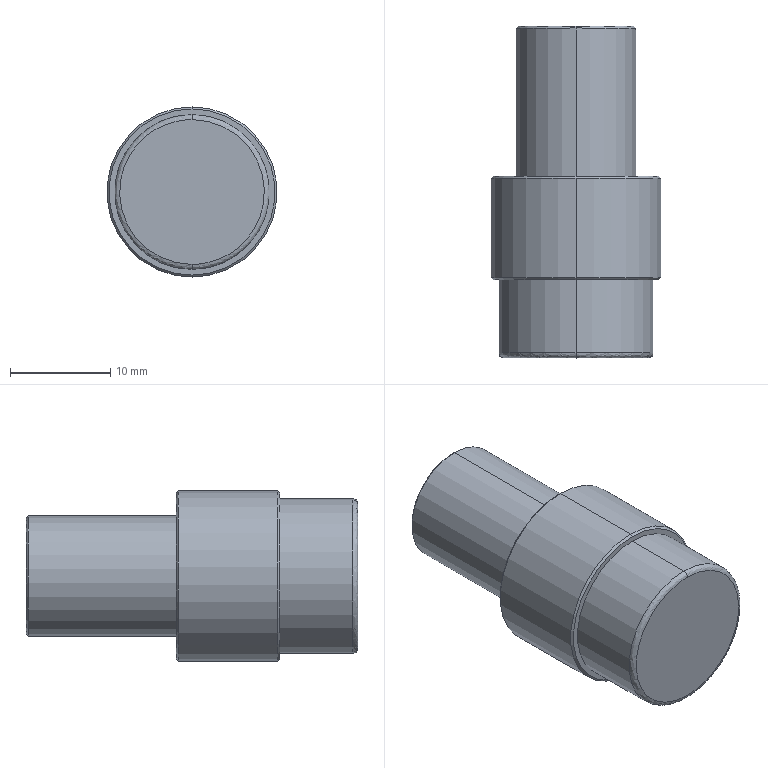Part | SolidWorks | features BaseBody 1 | 1 solid | 18 faces | box 17 x 33.14 x 17 mm | volume 5502 mm3 | cylinder 6 | cone 6 | plane 4 | spline 2 | commonest cylinder face diameters 12 x2 15.46 x2 17 x2
STEP:
#1=CARTESIAN_POINT('',(0.,0.5,-7.73));
#2=VERTEX_POINT('',#1);
#3=CARTESIAN_POINT('',(0.,0.5,7.73));
#4=VERTEX_POINT('',#3);
#5=CARTESIAN_POINT('',(0.,0.5,0.));
#6=DIRECTION('',(0.,1.,0.));
#7=DIRECTION('',(0.,0.,-1.));
#8=AXIS2_PLACEMENT_3D('',#5,#6,#7);
#9=CIRCLE('',#8,7.73);
#10=EDGE_CURVE('',#2,#4,#9,.T.);
#11=ORIENTED_EDGE('',*,*,#10,.F.);
#12=CARTESIAN_POINT('',(0.,0.,-7.23));
#13=VERTEX_POINT('',#12);
#14=CARTESIAN_POINT('',(0.,0.5,-7.23));
#15=DIRECTION('',(-1.,0.,0.));
#16=DIRECTION('',(0.,0.,-1.));
#17=AXIS2_PLACEMENT_3D('',#14,#15,#16);
#18=CIRCLE('',#17,0.5);
#19=EDGE_CURVE('',#2,#13,#18,.T.);
#20=ORIENTED_EDGE('',*,*,#19,.T.);
#21=CARTESIAN_POINT('',(0.,0.,7.23));
#22=VERTEX_POINT('',#21);
#23=CARTESIAN_POINT('',(0.,0.,-7.23));
#24=CARTESIAN_POINT('',(-14.46,0.,-7.23));
#25=CARTESIAN_POINT('',(-14.46,0.,7.23));
#26=CARTESIAN_POINT('',(0.,0.,7.23));
#27=(BOUNDED_CURVE()B_SPLINE_CURVE(3,(#23,#24,#25,#26),.UNSPECIFIED.,.F.,.T.)B_SPLINE_CURVE_WITH_KNOTS((4,4),(0.,1.),.UNSPECIFIED.)CURVE()GEOMETRIC_REPRESENTATION_ITEM()RATIONAL_B_SPLINE_CURVE((1.,0.3333,0.3333,1.))REPRESENTATION_ITEM(''));
#28=EDGE_CURVE('',#13,#22,#27,.T.);
#29=ORIENTED_EDGE('',*,*,#28,.T.);
#30=CARTESIAN_POINT('',(0.,0.5,7.23));
#31=DIRECTION('',(1.,0.,0.));
#32=DIRECTION('',(0.,0.,1.));
#33=AXIS2_PLACEMENT_3D('',#30,#31,#32);
#34=CIRCLE('',#33,0.5);
#35=EDGE_CURVE('',#4,#22,#34,.T.);
#36=ORIENTED_EDGE('',*,*,#35,.F.);
#37=EDGE_LOOP('',(#11,#20,#29,#36));
#38=FACE_OUTER_BOUND('',#37,.T.);
#39=CARTESIAN_POINT('',(0.,0.5,-7.73));
#40=CARTESIAN_POINT('',(-15.46,0.5,-7.73));
#41=CARTESIAN_POINT('',(-15.46,0.5,7.73));
#42=CARTESIAN_POINT('',(0.,0.5,7.73));
#43=CARTESIAN_POINT('',(0.,0.2071,-7.73));
#44=CARTESIAN_POINT('',(-15.46,0.2071,-7.73));
#45=CARTESIAN_POINT('',(-15.46,0.2071,7.73));
#46=CARTESIAN_POINT('',(0.,0.2071,7.73));
#47=CARTESIAN_POINT('',(0.,0.,-7.523));
#48=CARTESIAN_POINT('',(-15.046,0.,-7.523));
#49=CARTESIAN_POINT('',(-15.046,0.,7.523));
#50=CARTESIAN_POINT('',(0.,0.,7.523));
#51=CARTESIAN_POINT('',(0.,0.,-7.23));
#52=CARTESIAN_POINT('',(-14.46,0.,-7.23));
#53=CARTESIAN_POINT('',(-14.46,0.,7.23));
#54=CARTESIAN_POINT('',(0.,0.,7.23));
#55=(BOUNDED_SURFACE()B_SPLINE_SURFACE(3,3,((#39,#40,#41,#42),(#43,#44,#45,#46),(#47,#48,#49,#50),(#51,#52,#53,#54)),.UNSPECIFIED.,.F.,.F.,.F.)B_SPLINE_SURFACE_WITH_KNOTS((4,4),(4,4),(0.,1.),(0.,1.),.UNSPECIFIED.)GEOMETRIC_REPRESENTATION_ITEM()RATIONAL_B_SPLINE_SURFACE(((1.,0.3333,0.3333,1.),(0.8047,0.2682,0.2682,0.8047),(0.8047,0.2682,0.2682,0.8047),(1.,0.3333,0.3333,1.)))REPRESENTATION_ITEM('')SURFACE());
#56=ADVANCED_FACE('',(#38),#55,.T.);
#57=CARTESIAN_POINT('',(0.,32.94,-6.));
#58=VERTEX_POINT('',#57);
#59=CARTESIAN_POINT('',(0.,32.94,6.));
#60=VERTEX_POINT('',#59);
#61=CARTESIAN_POINT('',(0.,32.94,0.));
#62=DIRECTION('',(0.,-1.,0.));
#63=DIRECTION('',(0.,0.,-1.));
#64=AXIS2_PLACEMENT_3D('',#61,#62,#63);
#65=CIRCLE('',#64,6.);
#66=EDGE_CURVE('',#58,#60,#65,.T.);
#67=ORIENTED_EDGE('',*,*,#66,.T.);
#68=CARTESIAN_POINT('',(0.,18.14,6.));
#69=VERTEX_POINT('',#68);
#70=CARTESIAN_POINT('',(0.,33.14,6.));
#71=DIRECTION('',(0.,-1.,0.));
#72=VECTOR('',#71,1000.);
#73=LINE('',#70,#72);
#74=EDGE_CURVE('',#60,#69,#73,.T.);
#75=ORIENTED_EDGE('',*,*,#74,.T.);
#76=CARTESIAN_POINT('',(0.,18.14,-6.));
#77=VERTEX_POINT('',#76);
#78=CARTESIAN_POINT('',(0.,18.14,0.));
#79=DIRECTION('',(0.,1.,0.));
#80=DIRECTION('',(0.,0.,-1.));
#81=AXIS2_PLACEMENT_3D('',#78,#79,#80);
#82=CIRCLE('',#81,6.);
#83=EDGE_CURVE('',#69,#77,#82,.T.);
#84=ORIENTED_EDGE('',*,*,#83,.T.);
#85=CARTESIAN_POINT('',(0.,33.14,-6.));
#86=DIRECTION('',(0.,-1.,0.));
#87=VECTOR('',#86,1000.);
#88=LINE('',#85,#87);
#89=EDGE_CURVE('',#58,#77,#88,.T.);
#90=ORIENTED_EDGE('',*,*,#89,.F.);
#91=EDGE_LOOP('',(#67,#75,#84,#90));
#92=FACE_OUTER_BOUND('',#91,.T.);
#93=CARTESIAN_POINT('',(0.,33.14,0.));
#94=DIRECTION('',(0.,-1.,0.));
#95=DIRECTION('',(0.,0.,-1.));
#96=AXIS2_PLACEMENT_3D('',#93,#94,#95);
#97=CYLINDRICAL_SURFACE('',#96,6.);
#98=ADVANCED_FACE('',(#92),#97,.T.);
#99=CARTESIAN_POINT('',(0.,33.14,-5.8));
#100=VERTEX_POINT('',#99);
#101=CARTESIAN_POINT('',(0.,33.14,5.8));
#102=VERTEX_POINT('',#101);
#103=CARTESIAN_POINT('',(0.,33.14,0.));
#104=DIRECTION('',(0.,-1.,0.));
#105=DIRECTION('',(0.,0.,-1.));
#106=AXIS2_PLACEMENT_3D('',#103,#104,#105);
#107=CIRCLE('',#106,5.8);
#108=EDGE_CURVE('',#100,#102,#107,.T.);
#109=ORIENTED_EDGE('',*,*,#108,.T.);
#110=CARTESIAN_POINT('',(0.,32.94,6.));
#111=DIRECTION('',(0.,-0.7071,0.7071));
#112=VECTOR('',#111,1000.);
#113=LINE('',#110,#112);
#114=EDGE_CURVE('',#102,#60,#113,.T.);
#115=ORIENTED_EDGE('',*,*,#114,.T.);
#116=ORIENTED_EDGE('',*,*,#66,.F.);
#117=CARTESIAN_POINT('',(0.,32.94,-6.));
#118=DIRECTION('',(0.,-0.7071,-0.7071));
#119=VECTOR('',#118,1000.);
#120=LINE('',#117,#119);
#121=EDGE_CURVE('',#100,#58,#120,.T.);
#122=ORIENTED_EDGE('',*,*,#121,.F.);
#123=EDGE_LOOP('',(#109,#115,#116,#122));
#124=FACE_OUTER_BOUND('',#123,.T.);
#125=CARTESIAN_POINT('',(0.,32.94,0.));
#126=DIRECTION('',(0.,-1.,0.));
#127=DIRECTION('',(0.,0.,-1.));
#128=AXIS2_PLACEMENT_3D('',#125,#126,#127);
#129=CONICAL_SURFACE('',#128,6.,0.7854);
#130=ADVANCED_FACE('',(#124),#129,.T.);
#131=CARTESIAN_POINT('',(0.,18.14,8.3));
#132=VERTEX_POINT('',#131);
#133=CARTESIAN_POINT('',(0.,18.14,-8.3));
#134=VERTEX_POINT('',#133);
#135=CARTESIAN_POINT('',(0.,18.14,0.));
#136=DIRECTION('',(0.,1.,0.));
#137=DIRECTION('',(0.,0.,-1.));
#138=AXIS2_PLACEMENT_3D('',#135,#136,#137);
#139=CIRCLE('',#138,8.3);
#140=EDGE_CURVE('',#132,#134,#139,.T.);
#141=ORIENTED_EDGE('',*,*,#140,.F.);
#142=CARTESIAN_POINT('',(0.,17.94,8.5));
#143=VERTEX_POINT('',#142);
#144=CARTESIAN_POINT('',(0.,17.94,8.5));
#145=DIRECTION('',(0.,-0.7071,0.7071));
#146=VECTOR('',#145,1000.);
#147=LINE('',#144,#146);
#148=EDGE_CURVE('',#132,#143,#147,.T.);
#149=ORIENTED_EDGE('',*,*,#148,.T.);
#150=CARTESIAN_POINT('',(0.,17.94,-8.5));
#151=VERTEX_POINT('',#150);
#152=CARTESIAN_POINT('',(0.,17.94,0.));
#153=DIRECTION('',(0.,1.,0.));
#154=DIRECTION('',(0.,0.,-1.));
#155=AXIS2_PLACEMENT_3D('',#152,#153,#154);
#156=CIRCLE('',#155,8.5);
#157=EDGE_CURVE('',#143,#151,#156,.T.);
#158=ORIENTED_EDGE('',*,*,#157,.T.);
#159=CARTESIAN_POINT('',(0.,17.94,-8.5));
#160=DIRECTION('',(0.,-0.7071,-0.7071));
#161=VECTOR('',#160,1000.);
#162=LINE('',#159,#161);
#163=EDGE_CURVE('',#134,#151,#162,.T.);
#164=ORIENTED_EDGE('',*,*,#163,.F.);
#165=EDGE_LOOP('',(#141,#149,#158,#164));
#166=FACE_OUTER_BOUND('',#165,.T.);
#167=CARTESIAN_POINT('',(0.,17.94,0.));
#168=DIRECTION('',(0.,-1.,0.));
#169=DIRECTION('',(0.,0.,-1.));
#170=AXIS2_PLACEMENT_3D('',#167,#168,#169);
#171=CONICAL_SURFACE('',#170,8.5,0.7854);
#172=ADVANCED_FACE('',(#166),#171,.T.);
#173=ORIENTED_EDGE('',*,*,#157,.F.);
#174=CARTESIAN_POINT('',(0.,8.,8.5));
#175=VERTEX_POINT('',#174);
#176=CARTESIAN_POINT('',(0.,18.14,8.5));
#177=DIRECTION('',(0.,-1.,0.));
#178=VECTOR('',#177,1000.);
#179=LINE('',#176,#178);
#180=EDGE_CURVE('',#143,#175,#179,.T.);
#181=ORIENTED_EDGE('',*,*,#180,.T.);
#182=CARTESIAN_POINT('',(0.,8.,-8.5));
#183=VERTEX_POINT('',#182);
#184=CARTESIAN_POINT('',(0.,8.,0.));
#185=DIRECTION('',(0.,1.,0.));
#186=DIRECTION('',(0.,0.,-1.));
#187=AXIS2_PLACEMENT_3D('',#184,#185,#186);
#188=CIRCLE('',#187,8.5);
#189=EDGE_CURVE('',#175,#183,#188,.T.);
#190=ORIENTED_EDGE('',*,*,#189,.T.);
#191=CARTESIAN_POINT('',(0.,18.14,-8.5));
#192=DIRECTION('',(0.,-1.,0.));
#193=VECTOR('',#192,1000.);
#194=LINE('',#191,#193);
#195=EDGE_CURVE('',#151,#183,#194,.T.);
#196=ORIENTED_EDGE('',*,*,#195,.F.);
#197=EDGE_LOOP('',(#173,#181,#190,#196));
#198=FACE_OUTER_BOUND('',#197,.T.);
#199=CARTESIAN_POINT('',(0.,18.14,0.));
#200=DIRECTION('',(0.,-1.,0.));
#201=DIRECTION('',(0.,0.,-1.));
#202=AXIS2_PLACEMENT_3D('',#199,#200,#201);
#203=CYLINDRICAL_SURFACE('',#202,8.5);
#204=ADVANCED_FACE('',(#198),#203,.T.);
#205=CARTESIAN_POINT('',(0.,7.8,8.3));
#206=VERTEX_POINT('',#205);
#207=CARTESIAN_POINT('',(0.,7.8,-8.3));
#208=VERTEX_POINT('',#207);
#209=CARTESIAN_POINT('',(0.,7.8,0.));
#210=DIRECTION('',(0.,1.,0.));
#211=DIRECTION('',(0.,0.,1.));
#212=AXIS2_PLACEMENT_3D('',#209,#210,#211);
#213=CIRCLE('',#212,8.3);
#214=EDGE_CURVE('',#206,#208,#213,.T.);
#215=ORIENTED_EDGE('',*,*,#214,.T.);
#216=CARTESIAN_POINT('',(0.,8.,-8.5));
#217=DIRECTION('',(0.,0.7071,-0.7071));
#218=VECTOR('',#217,1000.);
#219=LINE('',#216,#218);
#220=EDGE_CURVE('',#208,#183,#219,.T.);
#221=ORIENTED_EDGE('',*,*,#220,.T.);
#222=ORIENTED_EDGE('',*,*,#189,.F.);
#223=CARTESIAN_POINT('',(0.,8.,8.5));
#224=DIRECTION('',(0.,0.7071,0.7071));
#225=VECTOR('',#224,1000.);
#226=LINE('',#223,#225);
#227=EDGE_CURVE('',#206,#175,#226,.T.);
#228=ORIENTED_EDGE('',*,*,#227,.F.);
#229=EDGE_LOOP('',(#215,#221,#222,#228));
#230=FACE_OUTER_BOUND('',#229,.T.);
#231=CARTESIAN_POINT('',(0.,8.,0.));
#232=DIRECTION('',(0.,1.,0.));
#233=DIRECTION('',(0.,0.,1.));
#234=AXIS2_PLACEMENT_3D('',#231,#232,#233);
#235=CONICAL_SURFACE('',#234,8.5,0.7854);
#236=ADVANCED_FACE('',(#230),#235,.T.);
#237=CARTESIAN_POINT('',(0.,7.8,-7.73));
#238=VERTEX_POINT('',#237);
#239=CARTESIAN_POINT('',(0.,7.8,7.73));
#240=VERTEX_POINT('',#239);
#241=CARTESIAN_POINT('',(0.,7.8,0.));
#242=DIRECTION('',(0.,-1.,0.));
#243=DIRECTION('',(0.,0.,-1.));
#244=AXIS2_PLACEMENT_3D('',#241,#242,#243);
#245=CIRCLE('',#244,7.73);
#246=EDGE_CURVE('',#238,#240,#245,.T.);
#247=ORIENTED_EDGE('',*,*,#246,.T.);
#248=CARTESIAN_POINT('',(0.,7.8,7.73));
#249=DIRECTION('',(0.,-1.,0.));
#250=VECTOR('',#249,1000.);
#251=LINE('',#248,#250);
#252=EDGE_CURVE('',#240,#4,#251,.T.);
#253=ORIENTED_EDGE('',*,*,#252,.T.);
#254=CARTESIAN_POINT('',(0.,0.5,0.));
#255=DIRECTION('',(0.,1.,0.));
#256=DIRECTION('',(0.,0.,-1.));
#257=AXIS2_PLACEMENT_3D('',#254,#255,#256);
#258=CIRCLE('',#257,7.73);
#259=EDGE_CURVE('',#4,#2,#258,.T.);
#260=ORIENTED_EDGE('',*,*,#259,.T.);
#261=CARTESIAN_POINT('',(0.,7.8,-7.73));
#262=DIRECTION('',(0.,-1.,0.));
#263=VECTOR('',#262,1000.);
#264=LINE('',#261,#263);
#265=EDGE_CURVE('',#238,#2,#264,.T.);
#266=ORIENTED_EDGE('',*,*,#265,.F.);
#267=EDGE_LOOP('',(#247,#253,#260,#266));
#268=FACE_OUTER_BOUND('',#267,.T.);
#269=CARTESIAN_POINT('',(0.,7.8,0.));
#270=DIRECTION('',(0.,-1.,0.));
#271=DIRECTION('',(0.,0.,-1.));
#272=AXIS2_PLACEMENT_3D('',#269,#270,#271);
#273=CYLINDRICAL_SURFACE('',#272,7.73);
#274=ADVANCED_FACE('',(#268),#273,.T.);
#275=ORIENTED_EDGE('',*,*,#74,.F.);
#276=CARTESIAN_POINT('',(0.,32.94,0.));
#277=DIRECTION('',(0.,-1.,0.));
#278=DIRECTION('',(0.,0.,-1.));
#279=AXIS2_PLACEMENT_3D('',#276,#277,#278);
#280=CIRCLE('',#279,6.);
#281=EDGE_CURVE('',#60,#58,#280,.T.);
#282=ORIENTED_EDGE('',*,*,#281,.T.);
#283=ORIENTED_EDGE('',*,*,#89,.T.);
#284=CARTESIAN_POINT('',(0.,18.14,0.));
#285=DIRECTION('',(0.,1.,0.));
#286=DIRECTION('',(0.,0.,-1.));
#287=AXIS2_PLACEMENT_3D('',#284,#285,#286);
#288=CIRCLE('',#287,6.);
#289=EDGE_CURVE('',#77,#69,#288,.T.);
#290=ORIENTED_EDGE('',*,*,#289,.T.);
#291=EDGE_LOOP('',(#275,#282,#283,#290));
#292=FACE_OUTER_BOUND('',#291,.T.);
#293=CARTESIAN_POINT('',(0.,33.14,0.));
#294=DIRECTION('',(0.,-1.,0.));
#295=DIRECTION('',(0.,0.,-1.));
#296=AXIS2_PLACEMENT_3D('',#293,#294,#295);
#297=CYLINDRICAL_SURFACE('',#296,6.);
#298=ADVANCED_FACE('',(#292),#297,.T.);
#299=ORIENTED_EDGE('',*,*,#289,.F.);
#300=ORIENTED_EDGE('',*,*,#83,.F.);
#301=EDGE_LOOP('',(#299,#300));
#302=FACE_BOUND('',#301,.T.);
#303=CARTESIAN_POINT('',(0.,18.14,0.));
#304=DIRECTION('',(0.,1.,0.));
#305=DIRECTION('',(0.,0.,-1.));
#306=AXIS2_PLACEMENT_3D('',#303,#304,#305);
#307=CIRCLE('',#306,8.3);
#308=EDGE_CURVE('',#134,#132,#307,.T.);
#309=ORIENTED_EDGE('',*,*,#308,.T.);
#310=ORIENTED_EDGE('',*,*,#140,.T.);
#311=EDGE_LOOP('',(#309,#310));
#312=FACE_OUTER_BOUND('',#311,.T.);
#313=CARTESIAN_POINT('',(0.,18.14,0.));
#314=DIRECTION('',(0.,1.,0.));
#315=DIRECTION('',(0.,0.,1.));
#316=AXIS2_PLACEMENT_3D('',#313,#314,#315);
#317=PLANE('',#316);
#318=ADVANCED_FACE('',(#302,#312),#317,.T.);
#319=ORIENTED_EDGE('',*,*,#114,.F.);
#320=CARTESIAN_POINT('',(0.,33.14,0.));
#321=DIRECTION('',(0.,-1.,0.));
#322=DIRECTION('',(0.,0.,-1.));
#323=AXIS2_PLACEMENT_3D('',#320,#321,#322);
#324=CIRCLE('',#323,5.8);
#325=EDGE_CURVE('',#102,#100,#324,.T.);
#326=ORIENTED_EDGE('',*,*,#325,.T.);
#327=ORIENTED_EDGE('',*,*,#121,.T.);
#328=ORIENTED_EDGE('',*,*,#281,.F.);
#329=EDGE_LOOP('',(#319,#326,#327,#328));
#330=FACE_OUTER_BOUND('',#329,.T.);
#331=CARTESIAN_POINT('',(0.,32.94,0.));
#332=DIRECTION('',(0.,-1.,0.));
#333=DIRECTION('',(0.,0.,-1.));
#334=AXIS2_PLACEMENT_3D('',#331,#332,#333);
#335=CONICAL_SURFACE('',#334,6.,0.7854);
#336=ADVANCED_FACE('',(#330),#335,.T.);
#337=ORIENTED_EDGE('',*,*,#148,.F.);
#338=ORIENTED_EDGE('',*,*,#308,.F.);
#339=ORIENTED_EDGE('',*,*,#163,.T.);
#340=CARTESIAN_POINT('',(0.,17.94,0.));
#341=DIRECTION('',(0.,1.,0.));
#342=DIRECTION('',(0.,0.,-1.));
#343=AXIS2_PLACEMENT_3D('',#340,#341,#342);
#344=CIRCLE('',#343,8.5);
#345=EDGE_CURVE('',#151,#143,#344,.T.);
#346=ORIENTED_EDGE('',*,*,#345,.T.);
#347=EDGE_LOOP('',(#337,#338,#339,#346));
#348=FACE_OUTER_BOUND('',#347,.T.);
#349=CARTESIAN_POINT('',(0.,17.94,0.));
#350=DIRECTION('',(0.,-1.,0.));
#351=DIRECTION('',(0.,0.,-1.));
#352=AXIS2_PLACEMENT_3D('',#349,#350,#351);
#353=CONICAL_SURFACE('',#352,8.5,0.7854);
#354=ADVANCED_FACE('',(#348),#353,.T.);
#355=ORIENTED_EDGE('',*,*,#108,.F.);
#356=ORIENTED_EDGE('',*,*,#325,.F.);
#357=EDGE_LOOP('',(#355,#356));
#358=FACE_OUTER_BOUND('',#357,.T.);
#359=CARTESIAN_POINT('',(0.,33.14,0.));
#360=DIRECTION('',(0.,1.,0.));
#361=DIRECTION('',(0.,0.,1.));
#362=AXIS2_PLACEMENT_3D('',#359,#360,#361);
#363=PLANE('',#362);
#364=ADVANCED_FACE('',(#358),#363,.T.);
#365=ORIENTED_EDGE('',*,*,#180,.F.);
#366=ORIENTED_EDGE('',*,*,#345,.F.);
#367=ORIENTED_EDGE('',*,*,#195,.T.);
#368=CARTESIAN_POINT('',(0.,8.,0.));
#369=DIRECTION('',(0.,1.,0.));
#370=DIRECTION('',(0.,0.,-1.));
#371=AXIS2_PLACEMENT_3D('',#368,#369,#370);
#372=CIRCLE('',#371,8.5);
#373=EDGE_CURVE('',#183,#175,#372,.T.);
#374=ORIENTED_EDGE('',*,*,#373,.T.);
#375=EDGE_LOOP('',(#365,#366,#367,#374));
#376=FACE_OUTER_BOUND('',#375,.T.);
#377=CARTESIAN_POINT('',(0.,18.14,0.));
#378=DIRECTION('',(0.,-1.,0.));
#379=DIRECTION('',(0.,0.,-1.));
#380=AXIS2_PLACEMENT_3D('',#377,#378,#379);
#381=CYLINDRICAL_SURFACE('',#380,8.5);
#382=ADVANCED_FACE('',(#376),#381,.T.);
#383=ORIENTED_EDGE('',*,*,#220,.F.);
#384=CARTESIAN_POINT('',(0.,7.8,0.));
#385=DIRECTION('',(0.,1.,0.));
#386=DIRECTION('',(0.,0.,1.));
#387=AXIS2_PLACEMENT_3D('',#384,#385,#386);
#388=CIRCLE('',#387,8.3);
#389=EDGE_CURVE('',#208,#206,#388,.T.);
#390=ORIENTED_EDGE('',*,*,#389,.T.);
#391=ORIENTED_EDGE('',*,*,#227,.T.);
#392=ORIENTED_EDGE('',*,*,#373,.F.);
#393=EDGE_LOOP('',(#383,#390,#391,#392));
#394=FACE_OUTER_BOUND('',#393,.T.);
#395=CARTESIAN_POINT('',(0.,8.,0.));
#396=DIRECTION('',(0.,1.,0.));
#397=DIRECTION('',(0.,0.,1.));
#398=AXIS2_PLACEMENT_3D('',#395,#396,#397);
#399=CONICAL_SURFACE('',#398,8.5,0.7854);
#400=ADVANCED_FACE('',(#394),#399,.T.);
#401=ORIENTED_EDGE('',*,*,#246,.F.);
#402=CARTESIAN_POINT('',(0.,7.8,0.));
#403=DIRECTION('',(0.,-1.,0.));
#404=DIRECTION('',(0.,0.,-1.));
#405=AXIS2_PLACEMENT_3D('',#402,#403,#404);
#406=CIRCLE('',#405,7.73);
#407=EDGE_CURVE('',#240,#238,#406,.T.);
#408=ORIENTED_EDGE('',*,*,#407,.F.);
#409=EDGE_LOOP('',(#401,#408));
#410=FACE_BOUND('',#409,.T.);
#411=ORIENTED_EDGE('',*,*,#214,.F.);
#412=ORIENTED_EDGE('',*,*,#389,.F.);
#413=EDGE_LOOP('',(#411,#412));
#414=FACE_OUTER_BOUND('',#413,.T.);
#415=CARTESIAN_POINT('',(0.,7.8,0.));
#416=DIRECTION('',(0.,1.,0.));
#417=DIRECTION('',(0.,0.,1.));
#418=AXIS2_PLACEMENT_3D('',#415,#416,#417);
#419=PLANE('',#418);
#420=ADVANCED_FACE('',(#410,#414),#419,.F.);
#421=ORIENTED_EDGE('',*,*,#252,.F.);
#422=ORIENTED_EDGE('',*,*,#407,.T.);
#423=ORIENTED_EDGE('',*,*,#265,.T.);
#424=ORIENTED_EDGE('',*,*,#10,.T.);
#425=EDGE_LOOP('',(#421,#422,#423,#424));
#426=FACE_OUTER_BOUND('',#425,.T.);
#427=CARTESIAN_POINT('',(0.,7.8,0.));
#428=DIRECTION('',(0.,-1.,0.));
#429=DIRECTION('',(0.,0.,-1.));
#430=AXIS2_PLACEMENT_3D('',#427,#428,#429);
#431=CYLINDRICAL_SURFACE('',#430,7.73);
#432=ADVANCED_FACE('',(#426),#431,.T.);
#433=ORIENTED_EDGE('',*,*,#19,.F.);
#434=ORIENTED_EDGE('',*,*,#259,.F.);
#435=ORIENTED_EDGE('',*,*,#35,.T.);
#436=CARTESIAN_POINT('',(0.,0.,7.23));
#437=CARTESIAN_POINT('',(14.46,0.,7.23));
#438=CARTESIAN_POINT('',(14.46,0.,-7.23));
#439=CARTESIAN_POINT('',(0.,0.,-7.23));
#440=(BOUNDED_CURVE()B_SPLINE_CURVE(3,(#436,#437,#438,#439),.UNSPECIFIED.,.F.,.F.)B_SPLINE_CURVE_WITH_KNOTS((4,4),(0.,1.),.UNSPECIFIED.)CURVE()GEOMETRIC_REPRESENTATION_ITEM()RATIONAL_B_SPLINE_CURVE((1.,0.3333,0.3333,1.))REPRESENTATION_ITEM(''));
#441=EDGE_CURVE('',#22,#13,#440,.T.);
#442=ORIENTED_EDGE('',*,*,#441,.T.);
#443=EDGE_LOOP('',(#433,#434,#435,#442));
#444=FACE_OUTER_BOUND('',#443,.T.);
#445=CARTESIAN_POINT('',(0.,0.5,7.73));
#446=CARTESIAN_POINT('',(15.46,0.5,7.73));
#447=CARTESIAN_POINT('',(15.46,0.5,-7.73));
#448=CARTESIAN_POINT('',(0.,0.5,-7.73));
#449=CARTESIAN_POINT('',(0.,0.2071,7.73));
#450=CARTESIAN_POINT('',(15.46,0.2071,7.73));
#451=CARTESIAN_POINT('',(15.46,0.2071,-7.73));
#452=CARTESIAN_POINT('',(0.,0.2071,-7.73));
#453=CARTESIAN_POINT('',(0.,0.,7.523));
#454=CARTESIAN_POINT('',(15.046,0.,7.523));
#455=CARTESIAN_POINT('',(15.046,0.,-7.523));
#456=CARTESIAN_POINT('',(0.,0.,-7.523));
#457=CARTESIAN_POINT('',(0.,0.,7.23));
#458=CARTESIAN_POINT('',(14.46,0.,7.23));
#459=CARTESIAN_POINT('',(14.46,0.,-7.23));
#460=CARTESIAN_POINT('',(0.,0.,-7.23));
#461=(BOUNDED_SURFACE()B_SPLINE_SURFACE(3,3,((#445,#446,#447,#448),(#449,#450,#451,#452),(#453,#454,#455,#456),(#457,#458,#459,#460)),.UNSPECIFIED.,.F.,.F.,.F.)B_SPLINE_SURFACE_WITH_KNOTS((4,4),(4,4),(0.,1.),(0.,1.),.UNSPECIFIED.)GEOMETRIC_REPRESENTATION_ITEM()RATIONAL_B_SPLINE_SURFACE(((1.,0.3333,0.3333,1.),(0.8047,0.2682,0.2682,0.8047),(0.8047,0.2682,0.2682,0.8047),(1.,0.3333,0.3333,1.)))REPRESENTATION_ITEM('')SURFACE());
#462=ADVANCED_FACE('',(#444),#461,.T.);
#463=ORIENTED_EDGE('',*,*,#441,.F.);
#464=ORIENTED_EDGE('',*,*,#28,.F.);
#465=EDGE_LOOP('',(#463,#464));
#466=FACE_OUTER_BOUND('',#465,.T.);
#467=CARTESIAN_POINT('',(0.,0.,0.));
#468=DIRECTION('',(0.,1.,0.));
#469=DIRECTION('',(0.,0.,1.));
#470=AXIS2_PLACEMENT_3D('',#467,#468,#469);
#471=PLANE('',#470);
#472=ADVANCED_FACE('',(#466),#471,.F.);
#473=CLOSED_SHELL('',(#56,#98,#130,#172,#204,#236,#274,#298,#318,#336,#354,#364,#382,#400,#420,#432,#462,#472));
#474=MANIFOLD_SOLID_BREP('',#473);
#475=CARTESIAN_POINT('',(0.,0.,0.));
#476=DIRECTION('',(0.,0.,1.));
#477=DIRECTION('',(1.,0.,0.));
#478=AXIS2_PLACEMENT_3D('',#475,#476,#477);
#479=(LENGTH_UNIT()NAMED_UNIT(*)SI_UNIT(.MILLI.,.METRE.));
#480=UNCERTAINTY_MEASURE_WITH_UNIT(LENGTH_MEASURE(0.00001),#479,'','');
#481=(NAMED_UNIT(*)PLANE_ANGLE_UNIT()SI_UNIT($,.RADIAN.));
#482=(NAMED_UNIT(*)SI_UNIT($,.STERADIAN.)SOLID_ANGLE_UNIT());
#483=(GEOMETRIC_REPRESENTATION_CONTEXT(3)GLOBAL_UNCERTAINTY_ASSIGNED_CONTEXT((#480))GLOBAL_UNIT_ASSIGNED_CONTEXT((#479,#481,#482))REPRESENTATION_CONTEXT('',''));
#484=ADVANCED_BREP_SHAPE_REPRESENTATION('',(#474,#478),#483);